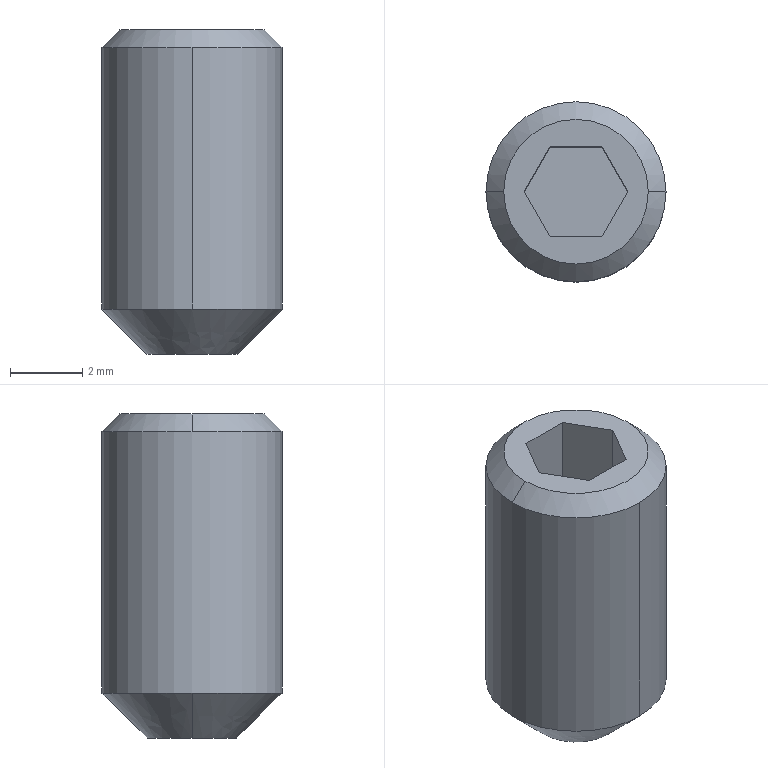Part | SolidWorks | features BaseBody 1 | 1 solid | 16 faces | box 5 x 5 x 9 mm | volume 134.698 mm3 | plane 8 | spline 6 | cylinder 2 | commonest cylinder face diameters 5 x2